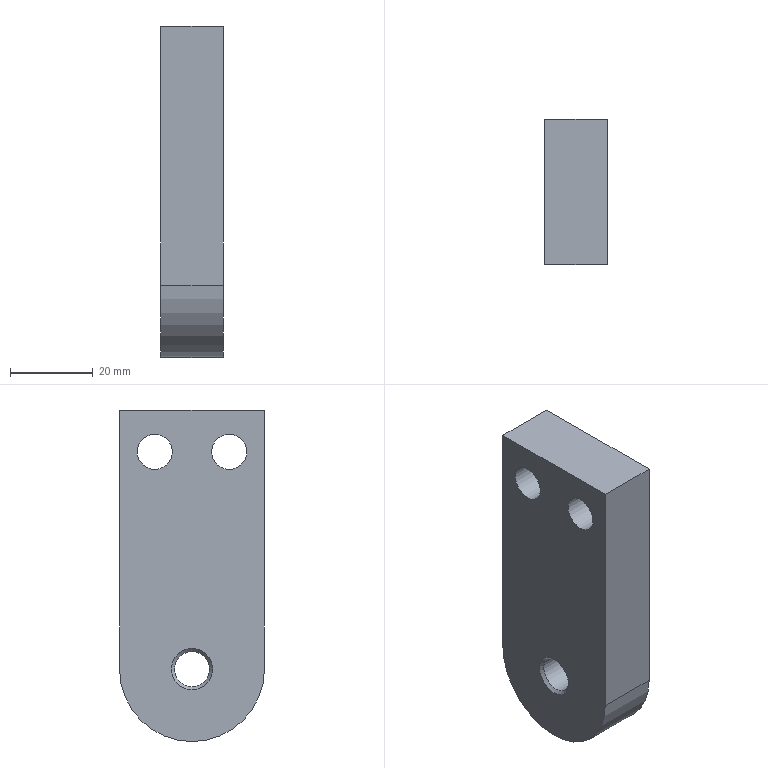Part | STEP file | Tube necking machine_id658_x_t | 1 solid | 15 faces | box 15 x 35 x 80 mm | volume 35904 mm3 | plane 7 | cylinder 6 | cone 2 | commonest cylinder face diameters 8.5 x3 14 x2 35 x1
STEP:
#1=CARTESIAN_POINT('',(0.,0.,0.));
#2=DIRECTION('',(0.,0.,1.));
#3=DIRECTION('',(1.,0.,0.));
#4=AXIS2_PLACEMENT_3D('',#1,#2,#3);
#5=CARTESIAN_POINT('',(215.,-121.,128.5));
#6=VERTEX_POINT('',#5);
#7=CARTESIAN_POINT('',(230.,-121.,128.5));
#8=VERTEX_POINT('',#7);
#9=CARTESIAN_POINT('',(230.,-121.,128.5));
#10=DIRECTION('',(1.,0.,0.));
#11=VECTOR('',#10,1.);
#12=LINE('',#9,#11);
#13=CARTESIAN_POINT('',(215.,-103.5,128.5));
#14=DIRECTION('',(1.,0.,0.));
#15=DIRECTION('',(0.,0.,-1.));
#16=AXIS2_PLACEMENT_3D('',#13,#14,#15);
#17=CYLINDRICAL_SURFACE('',#16,17.5);
#18=CARTESIAN_POINT('',(4.712,15.));
#19=DIRECTION('',(0.,1.));
#20=VECTOR('',#19,1.);
#21=LINE('',#18,#20);
#22=(GEOMETRIC_REPRESENTATION_CONTEXT(2)PARAMETRIC_REPRESENTATION_CONTEXT()REPRESENTATION_CONTEXT('',''));
#23=DEFINITIONAL_REPRESENTATION('',(#21),#22);
#24=PCURVE('',#17,#23);
#25=CARTESIAN_POINT('',(230.,-121.,191.));
#26=DIRECTION('',(0.,1.,0.));
#27=DIRECTION('',(0.,0.,1.));
#28=AXIS2_PLACEMENT_3D('',#25,#26,#27);
#29=PLANE('',#28);
#30=CARTESIAN_POINT('',(-62.5,0.));
#31=DIRECTION('',(0.,1.));
#32=VECTOR('',#31,1.);
#33=LINE('',#30,#32);
#34=(GEOMETRIC_REPRESENTATION_CONTEXT(2)PARAMETRIC_REPRESENTATION_CONTEXT()REPRESENTATION_CONTEXT('',''));
#35=DEFINITIONAL_REPRESENTATION('',(#33),#34);
#36=PCURVE('',#29,#35);
#37=SURFACE_CURVE('',#12,(#24,#36),.PCURVE_S1.);
#38=EDGE_CURVE('',#6,#8,#37,.T.);
#39=ORIENTED_EDGE('',*,*,#38,.F.);
#40=CARTESIAN_POINT('',(215.,-86.,128.5));
#41=VERTEX_POINT('',#40);
#42=CARTESIAN_POINT('',(215.,-103.5,128.5));
#43=DIRECTION('',(-1.,0.,0.));
#44=DIRECTION('',(0.,0.,-1.));
#45=AXIS2_PLACEMENT_3D('',#42,#43,#44);
#46=CIRCLE('',#45,17.5);
#47=CARTESIAN_POINT('',(12.566,0.));
#48=DIRECTION('',(-1.,0.));
#49=VECTOR('',#48,1.);
#50=LINE('',#47,#49);
#51=(GEOMETRIC_REPRESENTATION_CONTEXT(2)PARAMETRIC_REPRESENTATION_CONTEXT()REPRESENTATION_CONTEXT('',''));
#52=DEFINITIONAL_REPRESENTATION('',(#50),#51);
#53=PCURVE('',#17,#52);
#54=CARTESIAN_POINT('',(215.,0.,0.));
#55=DIRECTION('',(1.,0.,0.));
#56=DIRECTION('',(0.,0.,-1.));
#57=AXIS2_PLACEMENT_3D('',#54,#55,#56);
#58=PLANE('',#57);
#59=CARTESIAN_POINT('',(-111.,-103.5));
#60=CARTESIAN_POINT('',(-111.,-133.811));
#61=CARTESIAN_POINT('',(-137.25,-118.655));
#62=CARTESIAN_POINT('',(-163.5,-103.5));
#63=CARTESIAN_POINT('',(-137.25,-88.345));
#64=CARTESIAN_POINT('',(-111.,-73.189));
#65=CARTESIAN_POINT('',(-111.,-103.5));
#66=(BOUNDED_CURVE()B_SPLINE_CURVE(2,(#59,#60,#61,#62,#63,#64,#65),.UNSPECIFIED.,.T.,.F.)B_SPLINE_CURVE_WITH_KNOTS((1,2,2,2,2,1),(-2.094,0.,2.094,4.189,6.283,8.378),.UNSPECIFIED.)CURVE()GEOMETRIC_REPRESENTATION_ITEM()RATIONAL_B_SPLINE_CURVE((1.,0.5,1.,0.5,1.,0.5,1.))REPRESENTATION_ITEM(''));
#67=(GEOMETRIC_REPRESENTATION_CONTEXT(2)PARAMETRIC_REPRESENTATION_CONTEXT()REPRESENTATION_CONTEXT('',''));
#68=DEFINITIONAL_REPRESENTATION('',(#66),#67);
#69=PCURVE('',#58,#68);
#70=SURFACE_CURVE('',#46,(#53,#69),.PCURVE_S1.);
#71=EDGE_CURVE('',#41,#6,#70,.T.);
#72=ORIENTED_EDGE('',*,*,#71,.F.);
#73=CARTESIAN_POINT('',(230.,-86.,128.5));
#74=VERTEX_POINT('',#73);
#75=CARTESIAN_POINT('',(230.,-86.,128.5));
#76=DIRECTION('',(-1.,0.,0.));
#77=VECTOR('',#76,1.);
#78=LINE('',#75,#77);
#79=CARTESIAN_POINT('',(7.854,15.));
#80=DIRECTION('',(0.,-1.));
#81=VECTOR('',#80,1.);
#82=LINE('',#79,#81);
#83=(GEOMETRIC_REPRESENTATION_CONTEXT(2)PARAMETRIC_REPRESENTATION_CONTEXT()REPRESENTATION_CONTEXT('',''));
#84=DEFINITIONAL_REPRESENTATION('',(#82),#83);
#85=PCURVE('',#17,#84);
#86=CARTESIAN_POINT('',(230.,-86.,111.));
#87=DIRECTION('',(0.,-1.,0.));
#88=DIRECTION('',(0.,0.,-1.));
#89=AXIS2_PLACEMENT_3D('',#86,#87,#88);
#90=PLANE('',#89);
#91=CARTESIAN_POINT('',(-17.5,0.));
#92=DIRECTION('',(0.,-1.));
#93=VECTOR('',#92,1.);
#94=LINE('',#91,#93);
#95=(GEOMETRIC_REPRESENTATION_CONTEXT(2)PARAMETRIC_REPRESENTATION_CONTEXT()REPRESENTATION_CONTEXT('',''));
#96=DEFINITIONAL_REPRESENTATION('',(#94),#95);
#97=PCURVE('',#90,#96);
#98=SURFACE_CURVE('',#78,(#85,#97),.PCURVE_S1.);
#99=EDGE_CURVE('',#74,#41,#98,.T.);
#100=ORIENTED_EDGE('',*,*,#99,.F.);
#101=CARTESIAN_POINT('',(230.,-103.5,128.5));
#102=DIRECTION('',(1.,0.,0.));
#103=DIRECTION('',(0.,0.,-1.));
#104=AXIS2_PLACEMENT_3D('',#101,#102,#103);
#105=CIRCLE('',#104,17.5);
#106=CARTESIAN_POINT('',(0.,15.));
#107=DIRECTION('',(1.,0.));
#108=VECTOR('',#107,1.);
#109=LINE('',#106,#108);
#110=(GEOMETRIC_REPRESENTATION_CONTEXT(2)PARAMETRIC_REPRESENTATION_CONTEXT()REPRESENTATION_CONTEXT('',''));
#111=DEFINITIONAL_REPRESENTATION('',(#109),#110);
#112=PCURVE('',#17,#111);
#113=CARTESIAN_POINT('',(230.,0.,0.));
#114=DIRECTION('',(1.,0.,0.));
#115=DIRECTION('',(0.,0.,-1.));
#116=AXIS2_PLACEMENT_3D('',#113,#114,#115);
#117=PLANE('',#116);
#118=CARTESIAN_POINT('',(-128.5,-103.5));
#119=DIRECTION('',(1.,0.));
#120=AXIS2_PLACEMENT_2D('',#118,#119);
#121=CIRCLE('',#120,17.5);
#122=(GEOMETRIC_REPRESENTATION_CONTEXT(2)PARAMETRIC_REPRESENTATION_CONTEXT()REPRESENTATION_CONTEXT('',''));
#123=DEFINITIONAL_REPRESENTATION('',(#121),#122);
#124=PCURVE('',#117,#123);
#125=SURFACE_CURVE('',#105,(#112,#124),.PCURVE_S1.);
#126=EDGE_CURVE('',#8,#74,#125,.T.);
#127=ORIENTED_EDGE('',*,*,#126,.F.);
#128=EDGE_LOOP('',(#39,#72,#100,#127));
#129=FACE_BOUND('',#128,.T.);
#130=ADVANCED_FACE('',(#129),#17,.T.);
#131=CARTESIAN_POINT('',(215.,-121.,191.));
#132=VERTEX_POINT('',#131);
#133=CARTESIAN_POINT('',(215.,-121.,191.));
#134=DIRECTION('',(0.,0.,-1.));
#135=VECTOR('',#134,1.);
#136=LINE('',#133,#135);
#137=CARTESIAN_POINT('',(0.,-15.));
#138=DIRECTION('',(-1.,0.));
#139=VECTOR('',#138,1.);
#140=LINE('',#137,#139);
#141=(GEOMETRIC_REPRESENTATION_CONTEXT(2)PARAMETRIC_REPRESENTATION_CONTEXT()REPRESENTATION_CONTEXT('',''));
#142=DEFINITIONAL_REPRESENTATION('',(#140),#141);
#143=PCURVE('',#29,#142);
#144=CARTESIAN_POINT('',(-191.,-121.));
#145=DIRECTION('',(1.,0.));
#146=VECTOR('',#145,1.);
#147=LINE('',#144,#146);
#148=(GEOMETRIC_REPRESENTATION_CONTEXT(2)PARAMETRIC_REPRESENTATION_CONTEXT()REPRESENTATION_CONTEXT('',''));
#149=DEFINITIONAL_REPRESENTATION('',(#147),#148);
#150=PCURVE('',#58,#149);
#151=SURFACE_CURVE('',#136,(#143,#150),.PCURVE_S1.);
#152=EDGE_CURVE('',#132,#6,#151,.T.);
#153=ORIENTED_EDGE('',*,*,#152,.T.);
#154=ORIENTED_EDGE('',*,*,#38,.T.);
#155=CARTESIAN_POINT('',(230.,-121.,191.));
#156=VERTEX_POINT('',#155);
#157=CARTESIAN_POINT('',(230.,-121.,191.));
#158=DIRECTION('',(0.,0.,-1.));
#159=VECTOR('',#158,1.);
#160=LINE('',#157,#159);
#161=CARTESIAN_POINT('',(0.,0.));
#162=DIRECTION('',(-1.,0.));
#163=VECTOR('',#162,1.);
#164=LINE('',#161,#163);
#165=(GEOMETRIC_REPRESENTATION_CONTEXT(2)PARAMETRIC_REPRESENTATION_CONTEXT()REPRESENTATION_CONTEXT('',''));
#166=DEFINITIONAL_REPRESENTATION('',(#164),#165);
#167=PCURVE('',#29,#166);
#168=CARTESIAN_POINT('',(-191.,-121.));
#169=DIRECTION('',(1.,0.));
#170=VECTOR('',#169,1.);
#171=LINE('',#168,#170);
#172=(GEOMETRIC_REPRESENTATION_CONTEXT(2)PARAMETRIC_REPRESENTATION_CONTEXT()REPRESENTATION_CONTEXT('',''));
#173=DEFINITIONAL_REPRESENTATION('',(#171),#172);
#174=PCURVE('',#117,#173);
#175=SURFACE_CURVE('',#160,(#167,#174),.PCURVE_S1.);
#176=EDGE_CURVE('',#156,#8,#175,.T.);
#177=ORIENTED_EDGE('',*,*,#176,.F.);
#178=CARTESIAN_POINT('',(230.,-121.,191.));
#179=DIRECTION('',(-1.,0.,0.));
#180=VECTOR('',#179,1.);
#181=LINE('',#178,#180);
#182=CARTESIAN_POINT('',(0.,0.));
#183=DIRECTION('',(0.,-1.));
#184=VECTOR('',#183,1.);
#185=LINE('',#182,#184);
#186=(GEOMETRIC_REPRESENTATION_CONTEXT(2)PARAMETRIC_REPRESENTATION_CONTEXT()REPRESENTATION_CONTEXT('',''));
#187=DEFINITIONAL_REPRESENTATION('',(#185),#186);
#188=PCURVE('',#29,#187);
#189=CARTESIAN_POINT('',(230.,-86.,191.));
#190=DIRECTION('',(0.,0.,-1.));
#191=DIRECTION('',(-1.,0.,0.));
#192=AXIS2_PLACEMENT_3D('',#189,#190,#191);
#193=PLANE('',#192);
#194=CARTESIAN_POINT('',(0.,-35.));
#195=DIRECTION('',(1.,0.));
#196=VECTOR('',#195,1.);
#197=LINE('',#194,#196);
#198=(GEOMETRIC_REPRESENTATION_CONTEXT(2)PARAMETRIC_REPRESENTATION_CONTEXT()REPRESENTATION_CONTEXT('',''));
#199=DEFINITIONAL_REPRESENTATION('',(#197),#198);
#200=PCURVE('',#193,#199);
#201=SURFACE_CURVE('',#181,(#188,#200),.PCURVE_S1.);
#202=EDGE_CURVE('',#156,#132,#201,.T.);
#203=ORIENTED_EDGE('',*,*,#202,.T.);
#204=EDGE_LOOP('',(#153,#154,#177,#203));
#205=FACE_BOUND('',#204,.T.);
#206=ADVANCED_FACE('',(#205),#29,.F.);
#207=CARTESIAN_POINT('',(230.,-86.,191.));
#208=VERTEX_POINT('',#207);
#209=CARTESIAN_POINT('',(230.,-86.,111.));
#210=DIRECTION('',(0.,0.,1.));
#211=VECTOR('',#210,1.);
#212=LINE('',#209,#211);
#213=CARTESIAN_POINT('',(0.,0.));
#214=DIRECTION('',(-1.,0.));
#215=VECTOR('',#214,1.);
#216=LINE('',#213,#215);
#217=(GEOMETRIC_REPRESENTATION_CONTEXT(2)PARAMETRIC_REPRESENTATION_CONTEXT()REPRESENTATION_CONTEXT('',''));
#218=DEFINITIONAL_REPRESENTATION('',(#216),#217);
#219=PCURVE('',#90,#218);
#220=CARTESIAN_POINT('',(-111.,-86.));
#221=DIRECTION('',(-1.,0.));
#222=VECTOR('',#221,1.);
#223=LINE('',#220,#222);
#224=(GEOMETRIC_REPRESENTATION_CONTEXT(2)PARAMETRIC_REPRESENTATION_CONTEXT()REPRESENTATION_CONTEXT('',''));
#225=DEFINITIONAL_REPRESENTATION('',(#223),#224);
#226=PCURVE('',#117,#225);
#227=SURFACE_CURVE('',#212,(#219,#226),.PCURVE_S1.);
#228=EDGE_CURVE('',#74,#208,#227,.T.);
#229=ORIENTED_EDGE('',*,*,#228,.F.);
#230=ORIENTED_EDGE('',*,*,#99,.T.);
#231=CARTESIAN_POINT('',(215.,-86.,191.));
#232=VERTEX_POINT('',#231);
#233=CARTESIAN_POINT('',(215.,-86.,111.));
#234=DIRECTION('',(0.,0.,1.));
#235=VECTOR('',#234,1.);
#236=LINE('',#233,#235);
#237=CARTESIAN_POINT('',(0.,-15.));
#238=DIRECTION('',(-1.,0.));
#239=VECTOR('',#238,1.);
#240=LINE('',#237,#239);
#241=(GEOMETRIC_REPRESENTATION_CONTEXT(2)PARAMETRIC_REPRESENTATION_CONTEXT()REPRESENTATION_CONTEXT('',''));
#242=DEFINITIONAL_REPRESENTATION('',(#240),#241);
#243=PCURVE('',#90,#242);
#244=CARTESIAN_POINT('',(-111.,-86.));
#245=DIRECTION('',(-1.,0.));
#246=VECTOR('',#245,1.);
#247=LINE('',#244,#246);
#248=(GEOMETRIC_REPRESENTATION_CONTEXT(2)PARAMETRIC_REPRESENTATION_CONTEXT()REPRESENTATION_CONTEXT('',''));
#249=DEFINITIONAL_REPRESENTATION('',(#247),#248);
#250=PCURVE('',#58,#249);
#251=SURFACE_CURVE('',#236,(#243,#250),.PCURVE_S1.);
#252=EDGE_CURVE('',#41,#232,#251,.T.);
#253=ORIENTED_EDGE('',*,*,#252,.T.);
#254=CARTESIAN_POINT('',(230.,-86.,191.));
#255=DIRECTION('',(-1.,0.,0.));
#256=VECTOR('',#255,1.);
#257=LINE('',#254,#256);
#258=CARTESIAN_POINT('',(-80.,0.));
#259=DIRECTION('',(0.,-1.));
#260=VECTOR('',#259,1.);
#261=LINE('',#258,#260);
#262=(GEOMETRIC_REPRESENTATION_CONTEXT(2)PARAMETRIC_REPRESENTATION_CONTEXT()REPRESENTATION_CONTEXT('',''));
#263=DEFINITIONAL_REPRESENTATION('',(#261),#262);
#264=PCURVE('',#90,#263);
#265=CARTESIAN_POINT('',(0.,0.));
#266=DIRECTION('',(1.,0.));
#267=VECTOR('',#266,1.);
#268=LINE('',#265,#267);
#269=(GEOMETRIC_REPRESENTATION_CONTEXT(2)PARAMETRIC_REPRESENTATION_CONTEXT()REPRESENTATION_CONTEXT('',''));
#270=DEFINITIONAL_REPRESENTATION('',(#268),#269);
#271=PCURVE('',#193,#270);
#272=SURFACE_CURVE('',#257,(#264,#271),.PCURVE_S1.);
#273=EDGE_CURVE('',#208,#232,#272,.T.);
#274=ORIENTED_EDGE('',*,*,#273,.F.);
#275=EDGE_LOOP('',(#229,#230,#253,#274));
#276=FACE_BOUND('',#275,.T.);
#277=ADVANCED_FACE('',(#276),#90,.F.);
#278=CARTESIAN_POINT('',(215.,-86.,191.));
#279=DIRECTION('',(0.,-1.,0.));
#280=VECTOR('',#279,1.);
#281=LINE('',#278,#280);
#282=CARTESIAN_POINT('',(15.,0.));
#283=DIRECTION('',(0.,-1.));
#284=VECTOR('',#283,1.);
#285=LINE('',#282,#284);
#286=(GEOMETRIC_REPRESENTATION_CONTEXT(2)PARAMETRIC_REPRESENTATION_CONTEXT()REPRESENTATION_CONTEXT('',''));
#287=DEFINITIONAL_REPRESENTATION('',(#285),#286);
#288=PCURVE('',#193,#287);
#289=CARTESIAN_POINT('',(-191.,-86.));
#290=DIRECTION('',(0.,-1.));
#291=VECTOR('',#290,1.);
#292=LINE('',#289,#291);
#293=(GEOMETRIC_REPRESENTATION_CONTEXT(2)PARAMETRIC_REPRESENTATION_CONTEXT()REPRESENTATION_CONTEXT('',''));
#294=DEFINITIONAL_REPRESENTATION('',(#292),#293);
#295=PCURVE('',#58,#294);
#296=SURFACE_CURVE('',#281,(#288,#295),.PCURVE_S1.);
#297=EDGE_CURVE('',#232,#132,#296,.T.);
#298=ORIENTED_EDGE('',*,*,#297,.T.);
#299=ORIENTED_EDGE('',*,*,#202,.F.);
#300=CARTESIAN_POINT('',(230.,-86.,191.));
#301=DIRECTION('',(0.,-1.,0.));
#302=VECTOR('',#301,1.);
#303=LINE('',#300,#302);
#304=CARTESIAN_POINT('',(0.,0.));
#305=DIRECTION('',(0.,-1.));
#306=VECTOR('',#305,1.);
#307=LINE('',#304,#306);
#308=(GEOMETRIC_REPRESENTATION_CONTEXT(2)PARAMETRIC_REPRESENTATION_CONTEXT()REPRESENTATION_CONTEXT('',''));
#309=DEFINITIONAL_REPRESENTATION('',(#307),#308);
#310=PCURVE('',#193,#309);
#311=CARTESIAN_POINT('',(-191.,-86.));
#312=DIRECTION('',(0.,-1.));
#313=VECTOR('',#312,1.);
#314=LINE('',#311,#313);
#315=(GEOMETRIC_REPRESENTATION_CONTEXT(2)PARAMETRIC_REPRESENTATION_CONTEXT()REPRESENTATION_CONTEXT('',''));
#316=DEFINITIONAL_REPRESENTATION('',(#314),#315);
#317=PCURVE('',#117,#316);
#318=SURFACE_CURVE('',#303,(#310,#317),.PCURVE_S1.);
#319=EDGE_CURVE('',#208,#156,#318,.T.);
#320=ORIENTED_EDGE('',*,*,#319,.F.);
#321=ORIENTED_EDGE('',*,*,#273,.T.);
#322=EDGE_LOOP('',(#298,#299,#320,#321));
#323=FACE_BOUND('',#322,.T.);
#324=ADVANCED_FACE('',(#323),#193,.F.);
#325=CARTESIAN_POINT('',(230.,-94.5,188.));
#326=VERTEX_POINT('',#325);
#327=CARTESIAN_POINT('',(230.,-94.5,181.));
#328=DIRECTION('',(-1.,0.,0.));
#329=DIRECTION('',(0.,0.,1.));
#330=AXIS2_PLACEMENT_3D('',#327,#328,#329);
#331=CIRCLE('',#330,7.);
#332=CARTESIAN_POINT('',(-188.,-94.5));
#333=CARTESIAN_POINT('',(-188.,-82.376));
#334=CARTESIAN_POINT('',(-177.5,-88.438));
#335=CARTESIAN_POINT('',(-167.,-94.5));
#336=CARTESIAN_POINT('',(-177.5,-100.562));
#337=CARTESIAN_POINT('',(-188.,-106.624));
#338=CARTESIAN_POINT('',(-188.,-94.5));
#339=(BOUNDED_CURVE()B_SPLINE_CURVE(2,(#332,#333,#334,#335,#336,#337,#338),.UNSPECIFIED.,.T.,.F.)B_SPLINE_CURVE_WITH_KNOTS((1,2,2,2,2,1),(-2.094,0.,2.094,4.189,6.283,8.378),.UNSPECIFIED.)CURVE()GEOMETRIC_REPRESENTATION_ITEM()RATIONAL_B_SPLINE_CURVE((1.,0.5,1.,0.5,1.,0.5,1.))REPRESENTATION_ITEM(''));
#340=(GEOMETRIC_REPRESENTATION_CONTEXT(2)PARAMETRIC_REPRESENTATION_CONTEXT()REPRESENTATION_CONTEXT('',''));
#341=DEFINITIONAL_REPRESENTATION('',(#339),#340);
#342=PCURVE('',#117,#341);
#343=CARTESIAN_POINT('',(230.,-94.5,181.));
#344=DIRECTION('',(-1.,0.,0.));
#345=DIRECTION('',(0.,0.,1.));
#346=AXIS2_PLACEMENT_3D('',#343,#344,#345);
#347=CYLINDRICAL_SURFACE('',#346,7.);
#348=CARTESIAN_POINT('',(0.,0.));
#349=DIRECTION('',(1.,0.));
#350=VECTOR('',#349,1.);
#351=LINE('',#348,#350);
#352=(GEOMETRIC_REPRESENTATION_CONTEXT(2)PARAMETRIC_REPRESENTATION_CONTEXT()REPRESENTATION_CONTEXT('',''));
#353=DEFINITIONAL_REPRESENTATION('',(#351),#352);
#354=PCURVE('',#347,#353);
#355=SURFACE_CURVE('',#331,(#342,#354),.PCURVE_S1.);
#356=EDGE_CURVE('',#326,#326,#355,.T.);
#357=ORIENTED_EDGE('',*,*,#356,.T.);
#358=EDGE_LOOP('',(#357));
#359=FACE_BOUND('',#358,.T.);
#360=CARTESIAN_POINT('',(230.,-112.5,188.));
#361=VERTEX_POINT('',#360);
#362=CARTESIAN_POINT('',(230.,-112.5,181.));
#363=DIRECTION('',(-1.,0.,0.));
#364=DIRECTION('',(0.,0.,1.));
#365=AXIS2_PLACEMENT_3D('',#362,#363,#364);
#366=CIRCLE('',#365,7.);
#367=CARTESIAN_POINT('',(-188.,-112.5));
#368=CARTESIAN_POINT('',(-188.,-100.376));
#369=CARTESIAN_POINT('',(-177.5,-106.438));
#370=CARTESIAN_POINT('',(-167.,-112.5));
#371=CARTESIAN_POINT('',(-177.5,-118.562));
#372=CARTESIAN_POINT('',(-188.,-124.624));
#373=CARTESIAN_POINT('',(-188.,-112.5));
#374=(BOUNDED_CURVE()B_SPLINE_CURVE(2,(#367,#368,#369,#370,#371,#372,#373),.UNSPECIFIED.,.T.,.F.)B_SPLINE_CURVE_WITH_KNOTS((1,2,2,2,2,1),(-2.094,0.,2.094,4.189,6.283,8.378),.UNSPECIFIED.)CURVE()GEOMETRIC_REPRESENTATION_ITEM()RATIONAL_B_SPLINE_CURVE((1.,0.5,1.,0.5,1.,0.5,1.))REPRESENTATION_ITEM(''));
#375=(GEOMETRIC_REPRESENTATION_CONTEXT(2)PARAMETRIC_REPRESENTATION_CONTEXT()REPRESENTATION_CONTEXT('',''));
#376=DEFINITIONAL_REPRESENTATION('',(#374),#375);
#377=PCURVE('',#117,#376);
#378=CARTESIAN_POINT('',(230.,-112.5,181.));
#379=DIRECTION('',(-1.,0.,0.));
#380=DIRECTION('',(0.,0.,1.));
#381=AXIS2_PLACEMENT_3D('',#378,#379,#380);
#382=CYLINDRICAL_SURFACE('',#381,7.);
#383=CARTESIAN_POINT('',(0.,0.));
#384=DIRECTION('',(1.,0.));
#385=VECTOR('',#384,1.);
#386=LINE('',#383,#385);
#387=(GEOMETRIC_REPRESENTATION_CONTEXT(2)PARAMETRIC_REPRESENTATION_CONTEXT()REPRESENTATION_CONTEXT('',''));
#388=DEFINITIONAL_REPRESENTATION('',(#386),#387);
#389=PCURVE('',#382,#388);
#390=SURFACE_CURVE('',#366,(#377,#389),.PCURVE_S1.);
#391=EDGE_CURVE('',#361,#361,#390,.T.);
#392=ORIENTED_EDGE('',*,*,#391,.T.);
#393=EDGE_LOOP('',(#392));
#394=FACE_BOUND('',#393,.T.);
#395=CARTESIAN_POINT('',(230.,-103.5,123.5));
#396=VERTEX_POINT('',#395);
#397=CARTESIAN_POINT('',(230.,-103.5,128.5));
#398=DIRECTION('',(-1.,0.,0.));
#399=DIRECTION('',(0.,0.,-1.));
#400=AXIS2_PLACEMENT_3D('',#397,#398,#399);
#401=CIRCLE('',#400,5.);
#402=CARTESIAN_POINT('',(-123.5,-103.5));
#403=CARTESIAN_POINT('',(-123.5,-112.16));
#404=CARTESIAN_POINT('',(-131.,-107.83));
#405=CARTESIAN_POINT('',(-138.5,-103.5));
#406=CARTESIAN_POINT('',(-131.,-99.17));
#407=CARTESIAN_POINT('',(-123.5,-94.84));
#408=CARTESIAN_POINT('',(-123.5,-103.5));
#409=(BOUNDED_CURVE()B_SPLINE_CURVE(2,(#402,#403,#404,#405,#406,#407,#408),.UNSPECIFIED.,.T.,.F.)B_SPLINE_CURVE_WITH_KNOTS((1,2,2,2,2,1),(-2.094,0.,2.094,4.189,6.283,8.378),.UNSPECIFIED.)CURVE()GEOMETRIC_REPRESENTATION_ITEM()RATIONAL_B_SPLINE_CURVE((1.,0.5,1.,0.5,1.,0.5,1.))REPRESENTATION_ITEM(''));
#410=(GEOMETRIC_REPRESENTATION_CONTEXT(2)PARAMETRIC_REPRESENTATION_CONTEXT()REPRESENTATION_CONTEXT('',''));
#411=DEFINITIONAL_REPRESENTATION('',(#409),#410);
#412=PCURVE('',#117,#411);
#413=CARTESIAN_POINT('',(230.,-103.5,128.5));
#414=DIRECTION('',(1.,0.,0.));
#415=DIRECTION('',(0.,0.,-1.));
#416=AXIS2_PLACEMENT_3D('',#413,#414,#415);
#417=CONICAL_SURFACE('',#416,5.,0.7854);
#418=CARTESIAN_POINT('',(6.283,0.));
#419=DIRECTION('',(-1.,0.));
#420=VECTOR('',#419,1.);
#421=LINE('',#418,#420);
#422=(GEOMETRIC_REPRESENTATION_CONTEXT(2)PARAMETRIC_REPRESENTATION_CONTEXT()REPRESENTATION_CONTEXT('',''));
#423=DEFINITIONAL_REPRESENTATION('',(#421),#422);
#424=PCURVE('',#417,#423);
#425=SURFACE_CURVE('',#401,(#412,#424),.PCURVE_S1.);
#426=EDGE_CURVE('',#396,#396,#425,.T.);
#427=ORIENTED_EDGE('',*,*,#426,.T.);
#428=EDGE_LOOP('',(#427));
#429=FACE_BOUND('',#428,.T.);
#430=ORIENTED_EDGE('',*,*,#176,.T.);
#431=ORIENTED_EDGE('',*,*,#126,.T.);
#432=ORIENTED_EDGE('',*,*,#228,.T.);
#433=ORIENTED_EDGE('',*,*,#319,.T.);
#434=EDGE_LOOP('',(#430,#431,#432,#433));
#435=FACE_BOUND('',#434,.T.);
#436=ADVANCED_FACE('',(#359,#394,#429,#435),#117,.T.);
#437=CARTESIAN_POINT('',(215.,-94.5,176.75));
#438=VERTEX_POINT('',#437);
#439=CARTESIAN_POINT('',(215.,-94.5,185.25));
#440=VERTEX_POINT('',#439);
#441=CARTESIAN_POINT('',(215.,-94.5,181.));
#442=DIRECTION('',(1.,0.,0.));
#443=DIRECTION('',(0.,0.,-1.));
#444=AXIS2_PLACEMENT_3D('',#441,#442,#443);
#445=CIRCLE('',#444,4.25);
#446=CARTESIAN_POINT('',(-181.,-94.5));
#447=DIRECTION('',(1.,0.));
#448=AXIS2_PLACEMENT_2D('',#446,#447);
#449=CIRCLE('',#448,4.25);
#450=(GEOMETRIC_REPRESENTATION_CONTEXT(2)PARAMETRIC_REPRESENTATION_CONTEXT()REPRESENTATION_CONTEXT('',''));
#451=DEFINITIONAL_REPRESENTATION('',(#449),#450);
#452=PCURVE('',#58,#451);
#453=CARTESIAN_POINT('',(185.169,-94.5,181.));
#454=DIRECTION('',(-1.,0.,0.));
#455=DIRECTION('',(0.,0.,1.));
#456=AXIS2_PLACEMENT_3D('',#453,#454,#455);
#457=CYLINDRICAL_SURFACE('',#456,4.25);
#458=CARTESIAN_POINT('',(3.142,-29.831));
#459=DIRECTION('',(-1.,0.));
#460=VECTOR('',#459,1.);
#461=LINE('',#458,#460);
#462=(GEOMETRIC_REPRESENTATION_CONTEXT(2)PARAMETRIC_REPRESENTATION_CONTEXT()REPRESENTATION_CONTEXT('',''));
#463=DEFINITIONAL_REPRESENTATION('',(#461),#462);
#464=PCURVE('',#457,#463);
#465=SURFACE_CURVE('',#445,(#452,#464),.PCURVE_S1.);
#466=EDGE_CURVE('',#438,#440,#465,.T.);
#467=ORIENTED_EDGE('',*,*,#466,.T.);
#468=CARTESIAN_POINT('',(215.,-94.5,181.));
#469=DIRECTION('',(1.,0.,0.));
#470=DIRECTION('',(0.,0.,-1.));
#471=AXIS2_PLACEMENT_3D('',#468,#469,#470);
#472=CIRCLE('',#471,4.25);
#473=CARTESIAN_POINT('',(-181.,-94.5));
#474=DIRECTION('',(1.,0.));
#475=AXIS2_PLACEMENT_2D('',#473,#474);
#476=CIRCLE('',#475,4.25);
#477=(GEOMETRIC_REPRESENTATION_CONTEXT(2)PARAMETRIC_REPRESENTATION_CONTEXT()REPRESENTATION_CONTEXT('',''));
#478=DEFINITIONAL_REPRESENTATION('',(#476),#477);
#479=PCURVE('',#58,#478);
#480=CARTESIAN_POINT('',(9.425,-29.831));
#481=DIRECTION('',(-1.,0.));
#482=VECTOR('',#481,1.);
#483=LINE('',#480,#482);
#484=(GEOMETRIC_REPRESENTATION_CONTEXT(2)PARAMETRIC_REPRESENTATION_CONTEXT()REPRESENTATION_CONTEXT('',''));
#485=DEFINITIONAL_REPRESENTATION('',(#483),#484);
#486=PCURVE('',#457,#485);
#487=SURFACE_CURVE('',#472,(#479,#486),.PCURVE_S1.);
#488=EDGE_CURVE('',#440,#438,#487,.T.);
#489=ORIENTED_EDGE('',*,*,#488,.T.);
#490=EDGE_LOOP('',(#467,#489));
#491=FACE_BOUND('',#490,.T.);
#492=CARTESIAN_POINT('',(215.,-112.5,176.75));
#493=VERTEX_POINT('',#492);
#494=CARTESIAN_POINT('',(215.,-112.5,185.25));
#495=VERTEX_POINT('',#494);
#496=CARTESIAN_POINT('',(215.,-112.5,181.));
#497=DIRECTION('',(1.,0.,0.));
#498=DIRECTION('',(0.,0.,-1.));
#499=AXIS2_PLACEMENT_3D('',#496,#497,#498);
#500=CIRCLE('',#499,4.25);
#501=CARTESIAN_POINT('',(-181.,-112.5));
#502=DIRECTION('',(1.,0.));
#503=AXIS2_PLACEMENT_2D('',#501,#502);
#504=CIRCLE('',#503,4.25);
#505=(GEOMETRIC_REPRESENTATION_CONTEXT(2)PARAMETRIC_REPRESENTATION_CONTEXT()REPRESENTATION_CONTEXT('',''));
#506=DEFINITIONAL_REPRESENTATION('',(#504),#505);
#507=PCURVE('',#58,#506);
#508=CARTESIAN_POINT('',(185.169,-112.5,181.));
#509=DIRECTION('',(-1.,0.,0.));
#510=DIRECTION('',(0.,0.,1.));
#511=AXIS2_PLACEMENT_3D('',#508,#509,#510);
#512=CYLINDRICAL_SURFACE('',#511,4.25);
#513=CARTESIAN_POINT('',(3.142,-29.831));
#514=DIRECTION('',(-1.,0.));
#515=VECTOR('',#514,1.);
#516=LINE('',#513,#515);
#517=(GEOMETRIC_REPRESENTATION_CONTEXT(2)PARAMETRIC_REPRESENTATION_CONTEXT()REPRESENTATION_CONTEXT('',''));
#518=DEFINITIONAL_REPRESENTATION('',(#516),#517);
#519=PCURVE('',#512,#518);
#520=SURFACE_CURVE('',#500,(#507,#519),.PCURVE_S1.);
#521=EDGE_CURVE('',#493,#495,#520,.T.);
#522=ORIENTED_EDGE('',*,*,#521,.T.);
#523=CARTESIAN_POINT('',(215.,-112.5,181.));
#524=DIRECTION('',(1.,0.,0.));
#525=DIRECTION('',(0.,0.,-1.));
#526=AXIS2_PLACEMENT_3D('',#523,#524,#525);
#527=CIRCLE('',#526,4.25);
#528=CARTESIAN_POINT('',(-181.,-112.5));
#529=DIRECTION('',(1.,0.));
#530=AXIS2_PLACEMENT_2D('',#528,#529);
#531=CIRCLE('',#530,4.25);
#532=(GEOMETRIC_REPRESENTATION_CONTEXT(2)PARAMETRIC_REPRESENTATION_CONTEXT()REPRESENTATION_CONTEXT('',''));
#533=DEFINITIONAL_REPRESENTATION('',(#531),#532);
#534=PCURVE('',#58,#533);
#535=CARTESIAN_POINT('',(9.425,-29.831));
#536=DIRECTION('',(-1.,0.));
#537=VECTOR('',#536,1.);
#538=LINE('',#535,#537);
#539=(GEOMETRIC_REPRESENTATION_CONTEXT(2)PARAMETRIC_REPRESENTATION_CONTEXT()REPRESENTATION_CONTEXT('',''));
#540=DEFINITIONAL_REPRESENTATION('',(#538),#539);
#541=PCURVE('',#512,#540);
#542=SURFACE_CURVE('',#527,(#534,#541),.PCURVE_S1.);
#543=EDGE_CURVE('',#495,#493,#542,.T.);
#544=ORIENTED_EDGE('',*,*,#543,.T.);
#545=EDGE_LOOP('',(#522,#544));
#546=FACE_BOUND('',#545,.T.);
#547=CARTESIAN_POINT('',(215.,-103.5,123.5));
#548=VERTEX_POINT('',#547);
#549=CARTESIAN_POINT('',(215.,-103.5,128.5));
#550=DIRECTION('',(1.,0.,0.));
#551=DIRECTION('',(0.,0.,-1.));
#552=AXIS2_PLACEMENT_3D('',#549,#550,#551);
#553=CIRCLE('',#552,5.);
#554=CARTESIAN_POINT('',(-128.5,-103.5));
#555=DIRECTION('',(1.,0.));
#556=AXIS2_PLACEMENT_2D('',#554,#555);
#557=CIRCLE('',#556,5.);
#558=(GEOMETRIC_REPRESENTATION_CONTEXT(2)PARAMETRIC_REPRESENTATION_CONTEXT()REPRESENTATION_CONTEXT('',''));
#559=DEFINITIONAL_REPRESENTATION('',(#557),#558);
#560=PCURVE('',#58,#559);
#561=CARTESIAN_POINT('',(215.,-103.5,128.5));
#562=DIRECTION('',(-1.,0.,0.));
#563=DIRECTION('',(0.,0.,1.));
#564=AXIS2_PLACEMENT_3D('',#561,#562,#563);
#565=CONICAL_SURFACE('',#564,5.,0.7854);
#566=CARTESIAN_POINT('',(9.425,0.));
#567=DIRECTION('',(-1.,0.));
#568=VECTOR('',#567,1.);
#569=LINE('',#566,#568);
#570=(GEOMETRIC_REPRESENTATION_CONTEXT(2)PARAMETRIC_REPRESENTATION_CONTEXT()REPRESENTATION_CONTEXT('',''));
#571=DEFINITIONAL_REPRESENTATION('',(#569),#570);
#572=PCURVE('',#565,#571);
#573=SURFACE_CURVE('',#553,(#560,#572),.PCURVE_S1.);
#574=EDGE_CURVE('',#548,#548,#573,.T.);
#575=ORIENTED_EDGE('',*,*,#574,.T.);
#576=EDGE_LOOP('',(#575));
#577=FACE_BOUND('',#576,.T.);
#578=ORIENTED_EDGE('',*,*,#252,.F.);
#579=ORIENTED_EDGE('',*,*,#71,.T.);
#580=ORIENTED_EDGE('',*,*,#152,.F.);
#581=ORIENTED_EDGE('',*,*,#297,.F.);
#582=EDGE_LOOP('',(#578,#579,#580,#581));
#583=FACE_BOUND('',#582,.T.);
#584=ADVANCED_FACE('',(#491,#546,#577,#583),#58,.F.);
#585=CARTESIAN_POINT('',(215.75,-103.5,124.25));
#586=VERTEX_POINT('',#585);
#587=CARTESIAN_POINT('',(215.75,-103.5,128.5));
#588=DIRECTION('',(-1.,0.,0.));
#589=DIRECTION('',(0.,0.,-1.));
#590=AXIS2_PLACEMENT_3D('',#587,#588,#589);
#591=CIRCLE('',#590,4.25);
#592=CARTESIAN_POINT('',(230.,-103.5,128.5));
#593=DIRECTION('',(-1.,0.,0.));
#594=DIRECTION('',(0.,0.,1.));
#595=AXIS2_PLACEMENT_3D('',#592,#593,#594);
#596=CYLINDRICAL_SURFACE('',#595,4.25);
#597=CARTESIAN_POINT('',(3.142,14.25));
#598=DIRECTION('',(1.,0.));
#599=VECTOR('',#598,1.);
#600=LINE('',#597,#599);
#601=(GEOMETRIC_REPRESENTATION_CONTEXT(2)PARAMETRIC_REPRESENTATION_CONTEXT()REPRESENTATION_CONTEXT('',''));
#602=DEFINITIONAL_REPRESENTATION('',(#600),#601);
#603=PCURVE('',#596,#602);
#604=CARTESIAN_POINT('',(3.142,-0.75));
#605=DIRECTION('',(1.,0.));
#606=VECTOR('',#605,1.);
#607=LINE('',#604,#606);
#608=(GEOMETRIC_REPRESENTATION_CONTEXT(2)PARAMETRIC_REPRESENTATION_CONTEXT()REPRESENTATION_CONTEXT('',''));
#609=DEFINITIONAL_REPRESENTATION('',(#607),#608);
#610=PCURVE('',#565,#609);
#611=SURFACE_CURVE('',#591,(#603,#610),.PCURVE_S1.);
#612=EDGE_CURVE('',#586,#586,#611,.T.);
#613=ORIENTED_EDGE('',*,*,#612,.F.);
#614=CARTESIAN_POINT('',(229.25,-103.5,124.25));
#615=VERTEX_POINT('',#614);
#616=CARTESIAN_POINT('',(229.25,-103.5,124.25));
#617=CARTESIAN_POINT('',(215.75,-103.5,124.25));
#618=B_SPLINE_CURVE_WITH_KNOTS('',1,(#616,#617),.UNSPECIFIED.,.F.,.F.,(2,2),(0.75,14.25),.PIECEWISE_BEZIER_KNOTS.);
#619=CARTESIAN_POINT('',(3.142,0.));
#620=DIRECTION('',(0.,1.));
#621=VECTOR('',#620,1.);
#622=LINE('',#619,#621);
#623=(GEOMETRIC_REPRESENTATION_CONTEXT(2)PARAMETRIC_REPRESENTATION_CONTEXT()REPRESENTATION_CONTEXT('',''));
#624=DEFINITIONAL_REPRESENTATION('',(#622),#623);
#625=PCURVE('',#596,#624);
#626=CARTESIAN_POINT('',(9.425,0.));
#627=DIRECTION('',(0.,1.));
#628=VECTOR('',#627,1.);
#629=LINE('',#626,#628);
#630=(GEOMETRIC_REPRESENTATION_CONTEXT(2)PARAMETRIC_REPRESENTATION_CONTEXT()REPRESENTATION_CONTEXT('',''));
#631=DEFINITIONAL_REPRESENTATION('',(#629),#630);
#632=PCURVE('',#596,#631);
#633=SEAM_CURVE('',#618,(#625,#632),.PCURVE_S1.);
#634=EDGE_CURVE('',#615,#586,#633,.T.);
#635=ORIENTED_EDGE('',*,*,#634,.F.);
#636=CARTESIAN_POINT('',(229.25,-103.5,128.5));
#637=DIRECTION('',(1.,0.,0.));
#638=DIRECTION('',(0.,0.,-1.));
#639=AXIS2_PLACEMENT_3D('',#636,#637,#638);
#640=CIRCLE('',#639,4.25);
#641=CARTESIAN_POINT('',(9.425,0.75));
#642=DIRECTION('',(-1.,0.));
#643=VECTOR('',#642,1.);
#644=LINE('',#641,#643);
#645=(GEOMETRIC_REPRESENTATION_CONTEXT(2)PARAMETRIC_REPRESENTATION_CONTEXT()REPRESENTATION_CONTEXT('',''));
#646=DEFINITIONAL_REPRESENTATION('',(#644),#645);
#647=PCURVE('',#596,#646);
#648=CARTESIAN_POINT('',(0.,-0.75));
#649=DIRECTION('',(1.,0.));
#650=VECTOR('',#649,1.);
#651=LINE('',#648,#650);
#652=(GEOMETRIC_REPRESENTATION_CONTEXT(2)PARAMETRIC_REPRESENTATION_CONTEXT()REPRESENTATION_CONTEXT('',''));
#653=DEFINITIONAL_REPRESENTATION('',(#651),#652);
#654=PCURVE('',#417,#653);
#655=SURFACE_CURVE('',#640,(#647,#654),.PCURVE_S1.);
#656=EDGE_CURVE('',#615,#615,#655,.T.);
#657=ORIENTED_EDGE('',*,*,#656,.F.);
#658=ORIENTED_EDGE('',*,*,#634,.T.);
#659=EDGE_LOOP('',(#613,#635,#657,#658));
#660=FACE_BOUND('',#659,.F.);
#661=ADVANCED_FACE('',(#660),#596,.F.);
#662=ORIENTED_EDGE('',*,*,#656,.T.);
#663=CARTESIAN_POINT('',(229.25,-103.5,124.25));
#664=CARTESIAN_POINT('',(230.,-103.5,123.5));
#665=B_SPLINE_CURVE_WITH_KNOTS('',1,(#663,#664),.UNSPECIFIED.,.F.,.F.,(2,2),(-1.061,0.),.PIECEWISE_BEZIER_KNOTS.);
#666=CARTESIAN_POINT('',(6.283,0.));
#667=DIRECTION('',(0.,1.));
#668=VECTOR('',#667,1.);
#669=LINE('',#666,#668);
#670=(GEOMETRIC_REPRESENTATION_CONTEXT(2)PARAMETRIC_REPRESENTATION_CONTEXT()REPRESENTATION_CONTEXT('',''));
#671=DEFINITIONAL_REPRESENTATION('',(#669),#670);
#672=PCURVE('',#417,#671);
#673=CARTESIAN_POINT('',(0.,0.));
#674=DIRECTION('',(0.,1.));
#675=VECTOR('',#674,1.);
#676=LINE('',#673,#675);
#677=(GEOMETRIC_REPRESENTATION_CONTEXT(2)PARAMETRIC_REPRESENTATION_CONTEXT()REPRESENTATION_CONTEXT('',''));
#678=DEFINITIONAL_REPRESENTATION('',(#676),#677);
#679=PCURVE('',#417,#678);
#680=SEAM_CURVE('',#665,(#672,#679),.PCURVE_S1.);
#681=EDGE_CURVE('',#615,#396,#680,.T.);
#682=ORIENTED_EDGE('',*,*,#681,.T.);
#683=ORIENTED_EDGE('',*,*,#426,.T.);
#684=ORIENTED_EDGE('',*,*,#681,.F.);
#685=EDGE_LOOP('',(#662,#682,#683,#684));
#686=FACE_BOUND('',#685,.F.);
#687=ADVANCED_FACE('',(#686),#417,.F.);
#688=ORIENTED_EDGE('',*,*,#612,.T.);
#689=CARTESIAN_POINT('',(215.75,-103.5,124.25));
#690=CARTESIAN_POINT('',(215.,-103.5,123.5));
#691=B_SPLINE_CURVE_WITH_KNOTS('',1,(#689,#690),.UNSPECIFIED.,.F.,.F.,(2,2),(-1.061,0.),.PIECEWISE_BEZIER_KNOTS.);
#692=CARTESIAN_POINT('',(9.425,0.));
#693=DIRECTION('',(0.,1.));
#694=VECTOR('',#693,1.);
#695=LINE('',#692,#694);
#696=(GEOMETRIC_REPRESENTATION_CONTEXT(2)PARAMETRIC_REPRESENTATION_CONTEXT()REPRESENTATION_CONTEXT('',''));
#697=DEFINITIONAL_REPRESENTATION('',(#695),#696);
#698=PCURVE('',#565,#697);
#699=CARTESIAN_POINT('',(3.142,0.));
#700=DIRECTION('',(0.,1.));
#701=VECTOR('',#700,1.);
#702=LINE('',#699,#701);
#703=(GEOMETRIC_REPRESENTATION_CONTEXT(2)PARAMETRIC_REPRESENTATION_CONTEXT()REPRESENTATION_CONTEXT('',''));
#704=DEFINITIONAL_REPRESENTATION('',(#702),#703);
#705=PCURVE('',#565,#704);
#706=SEAM_CURVE('',#691,(#698,#705),.PCURVE_S1.);
#707=EDGE_CURVE('',#586,#548,#706,.T.);
#708=ORIENTED_EDGE('',*,*,#707,.T.);
#709=ORIENTED_EDGE('',*,*,#574,.T.);
#710=ORIENTED_EDGE('',*,*,#707,.F.);
#711=EDGE_LOOP('',(#688,#708,#709,#710));
#712=FACE_BOUND('',#711,.F.);
#713=ADVANCED_FACE('',(#712),#565,.F.);
#714=CARTESIAN_POINT('',(222.,-112.5,185.25));
#715=VERTEX_POINT('',#714);
#716=CARTESIAN_POINT('',(222.,-112.5,181.));
#717=DIRECTION('',(1.,0.,0.));
#718=DIRECTION('',(0.,0.,1.));
#719=AXIS2_PLACEMENT_3D('',#716,#717,#718);
#720=CIRCLE('',#719,4.25);
#721=CARTESIAN_POINT('',(6.283,-36.831));
#722=DIRECTION('',(-1.,0.));
#723=VECTOR('',#722,1.);
#724=LINE('',#721,#723);
#725=(GEOMETRIC_REPRESENTATION_CONTEXT(2)PARAMETRIC_REPRESENTATION_CONTEXT()REPRESENTATION_CONTEXT('',''));
#726=DEFINITIONAL_REPRESENTATION('',(#724),#725);
#727=PCURVE('',#512,#726);
#728=CARTESIAN_POINT('',(222.,-112.5,181.));
#729=DIRECTION('',(-1.,0.,0.));
#730=DIRECTION('',(0.,0.,1.));
#731=AXIS2_PLACEMENT_3D('',#728,#729,#730);
#732=PLANE('',#731);
#733=CARTESIAN_POINT('',(4.25,0.));
#734=CARTESIAN_POINT('',(4.25,-7.361));
#735=CARTESIAN_POINT('',(-2.125,-3.681));
#736=CARTESIAN_POINT('',(-8.5,0.));
#737=CARTESIAN_POINT('',(-2.125,3.681));
#738=CARTESIAN_POINT('',(4.25,7.361));
#739=CARTESIAN_POINT('',(4.25,0.));
#740=(BOUNDED_CURVE()B_SPLINE_CURVE(2,(#733,#734,#735,#736,#737,#738,#739),.UNSPECIFIED.,.T.,.F.)B_SPLINE_CURVE_WITH_KNOTS((1,2,2,2,2,1),(-2.094,0.,2.094,4.189,6.283,8.378),.UNSPECIFIED.)CURVE()GEOMETRIC_REPRESENTATION_ITEM()RATIONAL_B_SPLINE_CURVE((1.,0.5,1.,0.5,1.,0.5,1.))REPRESENTATION_ITEM(''));
#741=(GEOMETRIC_REPRESENTATION_CONTEXT(2)PARAMETRIC_REPRESENTATION_CONTEXT()REPRESENTATION_CONTEXT('',''));
#742=DEFINITIONAL_REPRESENTATION('',(#740),#741);
#743=PCURVE('',#732,#742);
#744=SURFACE_CURVE('',#720,(#727,#743),.PCURVE_S1.);
#745=EDGE_CURVE('',#715,#715,#744,.T.);
#746=ORIENTED_EDGE('',*,*,#745,.F.);
#747=CARTESIAN_POINT('',(222.,-112.5,185.25));
#748=CARTESIAN_POINT('',(215.,-112.5,185.25));
#749=B_SPLINE_CURVE_WITH_KNOTS('',1,(#747,#748),.UNSPECIFIED.,.F.,.F.,(2,2),(-36.831,-29.831),.PIECEWISE_BEZIER_KNOTS.);
#750=CARTESIAN_POINT('',(6.283,0.));
#751=DIRECTION('',(0.,1.));
#752=VECTOR('',#751,1.);
#753=LINE('',#750,#752);
#754=(GEOMETRIC_REPRESENTATION_CONTEXT(2)PARAMETRIC_REPRESENTATION_CONTEXT()REPRESENTATION_CONTEXT('',''));
#755=DEFINITIONAL_REPRESENTATION('',(#753),#754);
#756=PCURVE('',#512,#755);
#757=CARTESIAN_POINT('',(0.,0.));
#758=DIRECTION('',(0.,1.));
#759=VECTOR('',#758,1.);
#760=LINE('',#757,#759);
#761=(GEOMETRIC_REPRESENTATION_CONTEXT(2)PARAMETRIC_REPRESENTATION_CONTEXT()REPRESENTATION_CONTEXT('',''));
#762=DEFINITIONAL_REPRESENTATION('',(#760),#761);
#763=PCURVE('',#512,#762);
#764=SEAM_CURVE('',#749,(#756,#763),.PCURVE_S1.);
#765=EDGE_CURVE('',#715,#495,#764,.T.);
#766=ORIENTED_EDGE('',*,*,#765,.T.);
#767=ORIENTED_EDGE('',*,*,#543,.T.);
#768=ORIENTED_EDGE('',*,*,#521,.T.);
#769=ORIENTED_EDGE('',*,*,#765,.F.);
#770=EDGE_LOOP('',(#746,#766,#767,#768,#769));
#771=FACE_BOUND('',#770,.F.);
#772=ADVANCED_FACE('',(#771),#512,.F.);
#773=ORIENTED_EDGE('',*,*,#745,.F.);
#774=EDGE_LOOP('',(#773));
#775=FACE_BOUND('',#774,.T.);
#776=CARTESIAN_POINT('',(222.,-112.5,188.));
#777=VERTEX_POINT('',#776);
#778=CARTESIAN_POINT('',(222.,-112.5,181.));
#779=DIRECTION('',(1.,0.,0.));
#780=DIRECTION('',(0.,0.,1.));
#781=AXIS2_PLACEMENT_3D('',#778,#779,#780);
#782=CIRCLE('',#781,7.);
#783=CARTESIAN_POINT('',(7.,0.));
#784=CARTESIAN_POINT('',(7.,-12.124));
#785=CARTESIAN_POINT('',(-3.5,-6.062));
#786=CARTESIAN_POINT('',(-14.,0.));
#787=CARTESIAN_POINT('',(-3.5,6.062));
#788=CARTESIAN_POINT('',(7.,12.124));
#789=CARTESIAN_POINT('',(7.,0.));
#790=(BOUNDED_CURVE()B_SPLINE_CURVE(2,(#783,#784,#785,#786,#787,#788,#789),.UNSPECIFIED.,.T.,.F.)B_SPLINE_CURVE_WITH_KNOTS((1,2,2,2,2,1),(-2.094,0.,2.094,4.189,6.283,8.378),.UNSPECIFIED.)CURVE()GEOMETRIC_REPRESENTATION_ITEM()RATIONAL_B_SPLINE_CURVE((1.,0.5,1.,0.5,1.,0.5,1.))REPRESENTATION_ITEM(''));
#791=(GEOMETRIC_REPRESENTATION_CONTEXT(2)PARAMETRIC_REPRESENTATION_CONTEXT()REPRESENTATION_CONTEXT('',''));
#792=DEFINITIONAL_REPRESENTATION('',(#790),#791);
#793=PCURVE('',#732,#792);
#794=CARTESIAN_POINT('',(6.283,8.));
#795=DIRECTION('',(-1.,0.));
#796=VECTOR('',#795,1.);
#797=LINE('',#794,#796);
#798=(GEOMETRIC_REPRESENTATION_CONTEXT(2)PARAMETRIC_REPRESENTATION_CONTEXT()REPRESENTATION_CONTEXT('',''));
#799=DEFINITIONAL_REPRESENTATION('',(#797),#798);
#800=PCURVE('',#382,#799);
#801=SURFACE_CURVE('',#782,(#793,#800),.PCURVE_S1.);
#802=EDGE_CURVE('',#777,#777,#801,.T.);
#803=ORIENTED_EDGE('',*,*,#802,.T.);
#804=EDGE_LOOP('',(#803));
#805=FACE_BOUND('',#804,.T.);
#806=ADVANCED_FACE('',(#775,#805),#732,.F.);
#807=ORIENTED_EDGE('',*,*,#802,.T.);
#808=CARTESIAN_POINT('',(230.,-112.5,188.));
#809=CARTESIAN_POINT('',(222.,-112.5,188.));
#810=B_SPLINE_CURVE_WITH_KNOTS('',1,(#808,#809),.UNSPECIFIED.,.F.,.F.,(2,2),(0.,8.),.PIECEWISE_BEZIER_KNOTS.);
#811=CARTESIAN_POINT('',(0.,0.));
#812=DIRECTION('',(0.,1.));
#813=VECTOR('',#812,1.);
#814=LINE('',#811,#813);
#815=(GEOMETRIC_REPRESENTATION_CONTEXT(2)PARAMETRIC_REPRESENTATION_CONTEXT()REPRESENTATION_CONTEXT('',''));
#816=DEFINITIONAL_REPRESENTATION('',(#814),#815);
#817=PCURVE('',#382,#816);
#818=CARTESIAN_POINT('',(6.283,0.));
#819=DIRECTION('',(0.,1.));
#820=VECTOR('',#819,1.);
#821=LINE('',#818,#820);
#822=(GEOMETRIC_REPRESENTATION_CONTEXT(2)PARAMETRIC_REPRESENTATION_CONTEXT()REPRESENTATION_CONTEXT('',''));
#823=DEFINITIONAL_REPRESENTATION('',(#821),#822);
#824=PCURVE('',#382,#823);
#825=SEAM_CURVE('',#810,(#817,#824),.PCURVE_S1.);
#826=EDGE_CURVE('',#361,#777,#825,.T.);
#827=ORIENTED_EDGE('',*,*,#826,.F.);
#828=ORIENTED_EDGE('',*,*,#391,.T.);
#829=ORIENTED_EDGE('',*,*,#826,.T.);
#830=EDGE_LOOP('',(#807,#827,#828,#829));
#831=FACE_BOUND('',#830,.F.);
#832=ADVANCED_FACE('',(#831),#382,.F.);
#833=CARTESIAN_POINT('',(222.,-94.5,185.25));
#834=VERTEX_POINT('',#833);
#835=CARTESIAN_POINT('',(222.,-94.5,181.));
#836=DIRECTION('',(1.,0.,0.));
#837=DIRECTION('',(0.,0.,1.));
#838=AXIS2_PLACEMENT_3D('',#835,#836,#837);
#839=CIRCLE('',#838,4.25);
#840=CARTESIAN_POINT('',(6.283,-36.831));
#841=DIRECTION('',(-1.,0.));
#842=VECTOR('',#841,1.);
#843=LINE('',#840,#842);
#844=(GEOMETRIC_REPRESENTATION_CONTEXT(2)PARAMETRIC_REPRESENTATION_CONTEXT()REPRESENTATION_CONTEXT('',''));
#845=DEFINITIONAL_REPRESENTATION('',(#843),#844);
#846=PCURVE('',#457,#845);
#847=CARTESIAN_POINT('',(222.,-94.5,181.));
#848=DIRECTION('',(-1.,0.,0.));
#849=DIRECTION('',(0.,0.,1.));
#850=AXIS2_PLACEMENT_3D('',#847,#848,#849);
#851=PLANE('',#850);
#852=CARTESIAN_POINT('',(4.25,0.));
#853=CARTESIAN_POINT('',(4.25,-7.361));
#854=CARTESIAN_POINT('',(-2.125,-3.681));
#855=CARTESIAN_POINT('',(-8.5,0.));
#856=CARTESIAN_POINT('',(-2.125,3.681));
#857=CARTESIAN_POINT('',(4.25,7.361));
#858=CARTESIAN_POINT('',(4.25,0.));
#859=(BOUNDED_CURVE()B_SPLINE_CURVE(2,(#852,#853,#854,#855,#856,#857,#858),.UNSPECIFIED.,.T.,.F.)B_SPLINE_CURVE_WITH_KNOTS((1,2,2,2,2,1),(-2.094,0.,2.094,4.189,6.283,8.378),.UNSPECIFIED.)CURVE()GEOMETRIC_REPRESENTATION_ITEM()RATIONAL_B_SPLINE_CURVE((1.,0.5,1.,0.5,1.,0.5,1.))REPRESENTATION_ITEM(''));
#860=(GEOMETRIC_REPRESENTATION_CONTEXT(2)PARAMETRIC_REPRESENTATION_CONTEXT()REPRESENTATION_CONTEXT('',''));
#861=DEFINITIONAL_REPRESENTATION('',(#859),#860);
#862=PCURVE('',#851,#861);
#863=SURFACE_CURVE('',#839,(#846,#862),.PCURVE_S1.);
#864=EDGE_CURVE('',#834,#834,#863,.T.);
#865=ORIENTED_EDGE('',*,*,#864,.F.);
#866=CARTESIAN_POINT('',(222.,-94.5,185.25));
#867=CARTESIAN_POINT('',(215.,-94.5,185.25));
#868=B_SPLINE_CURVE_WITH_KNOTS('',1,(#866,#867),.UNSPECIFIED.,.F.,.F.,(2,2),(-36.831,-29.831),.PIECEWISE_BEZIER_KNOTS.);
#869=CARTESIAN_POINT('',(6.283,0.));
#870=DIRECTION('',(0.,1.));
#871=VECTOR('',#870,1.);
#872=LINE('',#869,#871);
#873=(GEOMETRIC_REPRESENTATION_CONTEXT(2)PARAMETRIC_REPRESENTATION_CONTEXT()REPRESENTATION_CONTEXT('',''));
#874=DEFINITIONAL_REPRESENTATION('',(#872),#873);
#875=PCURVE('',#457,#874);
#876=CARTESIAN_POINT('',(0.,0.));
#877=DIRECTION('',(0.,1.));
#878=VECTOR('',#877,1.);
#879=LINE('',#876,#878);
#880=(GEOMETRIC_REPRESENTATION_CONTEXT(2)PARAMETRIC_REPRESENTATION_CONTEXT()REPRESENTATION_CONTEXT('',''));
#881=DEFINITIONAL_REPRESENTATION('',(#879),#880);
#882=PCURVE('',#457,#881);
#883=SEAM_CURVE('',#868,(#875,#882),.PCURVE_S1.);
#884=EDGE_CURVE('',#834,#440,#883,.T.);
#885=ORIENTED_EDGE('',*,*,#884,.T.);
#886=ORIENTED_EDGE('',*,*,#488,.T.);
#887=ORIENTED_EDGE('',*,*,#466,.T.);
#888=ORIENTED_EDGE('',*,*,#884,.F.);
#889=EDGE_LOOP('',(#865,#885,#886,#887,#888));
#890=FACE_BOUND('',#889,.F.);
#891=ADVANCED_FACE('',(#890),#457,.F.);
#892=ORIENTED_EDGE('',*,*,#864,.F.);
#893=EDGE_LOOP('',(#892));
#894=FACE_BOUND('',#893,.T.);
#895=CARTESIAN_POINT('',(222.,-94.5,188.));
#896=VERTEX_POINT('',#895);
#897=CARTESIAN_POINT('',(222.,-94.5,181.));
#898=DIRECTION('',(1.,0.,0.));
#899=DIRECTION('',(0.,0.,1.));
#900=AXIS2_PLACEMENT_3D('',#897,#898,#899);
#901=CIRCLE('',#900,7.);
#902=CARTESIAN_POINT('',(7.,0.));
#903=CARTESIAN_POINT('',(7.,-12.124));
#904=CARTESIAN_POINT('',(-3.5,-6.062));
#905=CARTESIAN_POINT('',(-14.,0.));
#906=CARTESIAN_POINT('',(-3.5,6.062));
#907=CARTESIAN_POINT('',(7.,12.124));
#908=CARTESIAN_POINT('',(7.,0.));
#909=(BOUNDED_CURVE()B_SPLINE_CURVE(2,(#902,#903,#904,#905,#906,#907,#908),.UNSPECIFIED.,.T.,.F.)B_SPLINE_CURVE_WITH_KNOTS((1,2,2,2,2,1),(-2.094,0.,2.094,4.189,6.283,8.378),.UNSPECIFIED.)CURVE()GEOMETRIC_REPRESENTATION_ITEM()RATIONAL_B_SPLINE_CURVE((1.,0.5,1.,0.5,1.,0.5,1.))REPRESENTATION_ITEM(''));
#910=(GEOMETRIC_REPRESENTATION_CONTEXT(2)PARAMETRIC_REPRESENTATION_CONTEXT()REPRESENTATION_CONTEXT('',''));
#911=DEFINITIONAL_REPRESENTATION('',(#909),#910);
#912=PCURVE('',#851,#911);
#913=CARTESIAN_POINT('',(6.283,8.));
#914=DIRECTION('',(-1.,0.));
#915=VECTOR('',#914,1.);
#916=LINE('',#913,#915);
#917=(GEOMETRIC_REPRESENTATION_CONTEXT(2)PARAMETRIC_REPRESENTATION_CONTEXT()REPRESENTATION_CONTEXT('',''));
#918=DEFINITIONAL_REPRESENTATION('',(#916),#917);
#919=PCURVE('',#347,#918);
#920=SURFACE_CURVE('',#901,(#912,#919),.PCURVE_S1.);
#921=EDGE_CURVE('',#896,#896,#920,.T.);
#922=ORIENTED_EDGE('',*,*,#921,.T.);
#923=EDGE_LOOP('',(#922));
#924=FACE_BOUND('',#923,.T.);
#925=ADVANCED_FACE('',(#894,#924),#851,.F.);
#926=ORIENTED_EDGE('',*,*,#921,.T.);
#927=CARTESIAN_POINT('',(230.,-94.5,188.));
#928=CARTESIAN_POINT('',(222.,-94.5,188.));
#929=B_SPLINE_CURVE_WITH_KNOTS('',1,(#927,#928),.UNSPECIFIED.,.F.,.F.,(2,2),(0.,8.),.PIECEWISE_BEZIER_KNOTS.);
#930=CARTESIAN_POINT('',(0.,0.));
#931=DIRECTION('',(0.,1.));
#932=VECTOR('',#931,1.);
#933=LINE('',#930,#932);
#934=(GEOMETRIC_REPRESENTATION_CONTEXT(2)PARAMETRIC_REPRESENTATION_CONTEXT()REPRESENTATION_CONTEXT('',''));
#935=DEFINITIONAL_REPRESENTATION('',(#933),#934);
#936=PCURVE('',#347,#935);
#937=CARTESIAN_POINT('',(6.283,0.));
#938=DIRECTION('',(0.,1.));
#939=VECTOR('',#938,1.);
#940=LINE('',#937,#939);
#941=(GEOMETRIC_REPRESENTATION_CONTEXT(2)PARAMETRIC_REPRESENTATION_CONTEXT()REPRESENTATION_CONTEXT('',''));
#942=DEFINITIONAL_REPRESENTATION('',(#940),#941);
#943=PCURVE('',#347,#942);
#944=SEAM_CURVE('',#929,(#936,#943),.PCURVE_S1.);
#945=EDGE_CURVE('',#326,#896,#944,.T.);
#946=ORIENTED_EDGE('',*,*,#945,.F.);
#947=ORIENTED_EDGE('',*,*,#356,.T.);
#948=ORIENTED_EDGE('',*,*,#945,.T.);
#949=EDGE_LOOP('',(#926,#946,#947,#948));
#950=FACE_BOUND('',#949,.F.);
#951=ADVANCED_FACE('',(#950),#347,.F.);
#952=CLOSED_SHELL('',(#130,#206,#277,#324,#436,#584,#661,#687,#713,#772,#806,#832,#891,#925,#951));
#953=MANIFOLD_SOLID_BREP('',#952);
#954=(LENGTH_UNIT()NAMED_UNIT(*)SI_UNIT(.MILLI.,.METRE.));
#955=UNCERTAINTY_MEASURE_WITH_UNIT(LENGTH_MEASURE(0.000005),#954,'','');
#956=(NAMED_UNIT(*)PLANE_ANGLE_UNIT()SI_UNIT($,.RADIAN.));
#957=(NAMED_UNIT(*)SI_UNIT($,.STERADIAN.)SOLID_ANGLE_UNIT());
#958=(GEOMETRIC_REPRESENTATION_CONTEXT(3)GLOBAL_UNCERTAINTY_ASSIGNED_CONTEXT((#955))GLOBAL_UNIT_ASSIGNED_CONTEXT((#954,#956,#957))REPRESENTATION_CONTEXT('',''));
#959=ADVANCED_BREP_SHAPE_REPRESENTATION('',(#4,#953),#958);